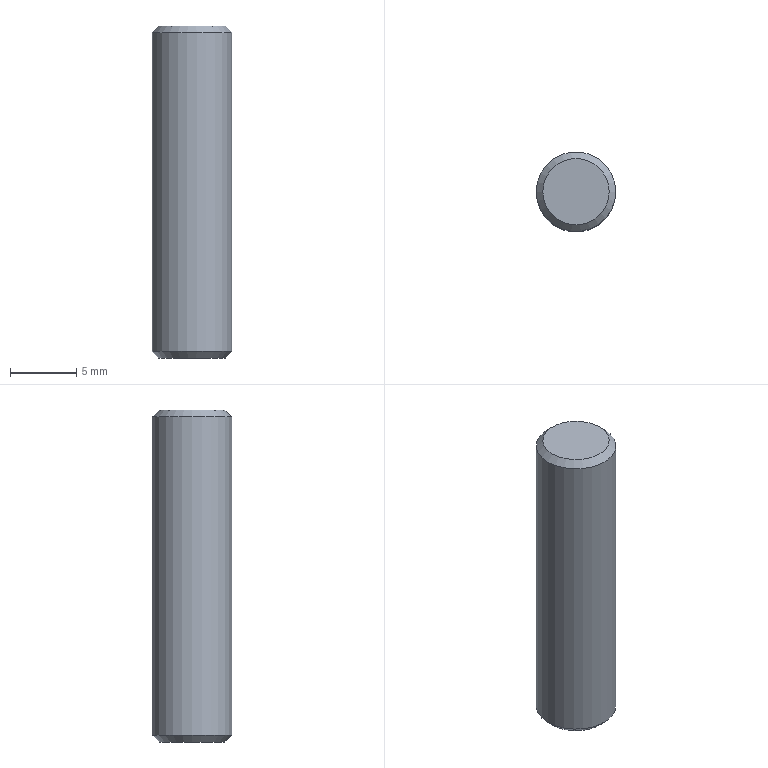Part | NX | features CHAMFER 2, DATUM_CSYS 2, EXTRUDE 1, SKETCH 1 | 1 solid | 5 faces | box 6 x 6 x 25 mm | volume 702.408 mm3 | plane 2 | cone 2 | cylinder 1 | commonest cylinder face diameters 6 x1
STEP:
#1=CARTESIAN_POINT('',(3.,0.,0.5));
#2=VERTEX_POINT('',#1);
#3=CARTESIAN_POINT('',(0.,0.,0.5));
#4=DIRECTION('',(0.,0.,1.));
#5=DIRECTION('',(1.,0.,0.));
#6=AXIS2_PLACEMENT_3D('',#3,#4,#5);
#7=CIRCLE('',#6,3.);
#8=EDGE_CURVE('',#2,#2,#7,.T.);
#9=ORIENTED_EDGE('',*,*,#8,.T.);
#10=EDGE_LOOP('',(#9));
#11=FACE_BOUND('',#10,.T.);
#12=CARTESIAN_POINT('',(3.,0.,24.5));
#13=VERTEX_POINT('',#12);
#14=CARTESIAN_POINT('',(0.,0.,24.5));
#15=DIRECTION('',(0.,0.,1.));
#16=DIRECTION('',(1.,0.,0.));
#17=AXIS2_PLACEMENT_3D('',#14,#15,#16);
#18=CIRCLE('',#17,3.);
#19=EDGE_CURVE('',#13,#13,#18,.F.);
#20=ORIENTED_EDGE('',*,*,#19,.T.);
#21=EDGE_LOOP('',(#20));
#22=FACE_BOUND('',#21,.T.);
#23=CARTESIAN_POINT('',(0.,0.,25.));
#24=DIRECTION('',(0.,0.,-1.));
#25=DIRECTION('',(-1.,0.,0.));
#26=AXIS2_PLACEMENT_3D('',#23,#24,#25);
#27=CYLINDRICAL_SURFACE('',#26,3.);
#28=ADVANCED_FACE('',(#11,#22),#27,.T.);
#29=CARTESIAN_POINT('',(2.5,0.,25.));
#30=VERTEX_POINT('',#29);
#31=CARTESIAN_POINT('',(0.,0.,25.));
#32=DIRECTION('',(0.,0.,1.));
#33=DIRECTION('',(1.,0.,0.));
#34=AXIS2_PLACEMENT_3D('',#31,#32,#33);
#35=CIRCLE('',#34,2.5);
#36=EDGE_CURVE('',#30,#30,#35,.T.);
#37=ORIENTED_EDGE('',*,*,#36,.T.);
#38=EDGE_LOOP('',(#37));
#39=FACE_BOUND('',#38,.T.);
#40=CARTESIAN_POINT('',(0.,0.,25.));
#41=DIRECTION('',(0.,0.,1.));
#42=DIRECTION('',(1.,0.,0.));
#43=AXIS2_PLACEMENT_3D('',#40,#41,#42);
#44=PLANE('',#43);
#45=ADVANCED_FACE('',(#39),#44,.T.);
#46=CARTESIAN_POINT('',(2.5,0.,0.));
#47=VERTEX_POINT('',#46);
#48=CARTESIAN_POINT('',(0.,0.,0.));
#49=DIRECTION('',(0.,0.,1.));
#50=DIRECTION('',(1.,0.,0.));
#51=AXIS2_PLACEMENT_3D('',#48,#49,#50);
#52=CIRCLE('',#51,2.5);
#53=EDGE_CURVE('',#47,#47,#52,.F.);
#54=ORIENTED_EDGE('',*,*,#53,.T.);
#55=EDGE_LOOP('',(#54));
#56=FACE_BOUND('',#55,.T.);
#57=CARTESIAN_POINT('',(0.,0.,0.));
#58=DIRECTION('',(0.,0.,1.));
#59=DIRECTION('',(1.,0.,0.));
#60=AXIS2_PLACEMENT_3D('',#57,#58,#59);
#61=PLANE('',#60);
#62=ADVANCED_FACE('',(#56),#61,.F.);
#63=ORIENTED_EDGE('',*,*,#19,.F.);
#64=EDGE_LOOP('',(#63));
#65=FACE_BOUND('',#64,.T.);
#66=ORIENTED_EDGE('',*,*,#36,.F.);
#67=EDGE_LOOP('',(#66));
#68=FACE_BOUND('',#67,.T.);
#69=CARTESIAN_POINT('',(0.,0.,25.));
#70=DIRECTION('',(0.,0.,-1.));
#71=DIRECTION('',(-1.,0.,0.));
#72=AXIS2_PLACEMENT_3D('',#69,#70,#71);
#73=CONICAL_SURFACE('',#72,2.5,0.7854);
#74=ADVANCED_FACE('',(#65,#68),#73,.T.);
#75=ORIENTED_EDGE('',*,*,#53,.F.);
#76=EDGE_LOOP('',(#75));
#77=FACE_BOUND('',#76,.T.);
#78=ORIENTED_EDGE('',*,*,#8,.F.);
#79=EDGE_LOOP('',(#78));
#80=FACE_BOUND('',#79,.T.);
#81=CARTESIAN_POINT('',(0.,0.,0.5));
#82=DIRECTION('',(0.,0.,1.));
#83=DIRECTION('',(1.,0.,0.));
#84=AXIS2_PLACEMENT_3D('',#81,#82,#83);
#85=CONICAL_SURFACE('',#84,3.,0.7854);
#86=ADVANCED_FACE('',(#77,#80),#85,.T.);
#87=CLOSED_SHELL('',(#28,#45,#62,#74,#86));
#88=MANIFOLD_SOLID_BREP('',#87);
#89=(LENGTH_UNIT()NAMED_UNIT(*)SI_UNIT(.MILLI.,.METRE.));
#90=UNCERTAINTY_MEASURE_WITH_UNIT(LENGTH_MEASURE(0.00001),#89,'','');
#91=(NAMED_UNIT(*)PLANE_ANGLE_UNIT()SI_UNIT($,.RADIAN.));
#92=(NAMED_UNIT(*)SI_UNIT($,.STERADIAN.)SOLID_ANGLE_UNIT());
#93=(GEOMETRIC_REPRESENTATION_CONTEXT(3)GLOBAL_UNCERTAINTY_ASSIGNED_CONTEXT((#90))GLOBAL_UNIT_ASSIGNED_CONTEXT((#89,#91,#92))REPRESENTATION_CONTEXT('',''));
#94=ADVANCED_BREP_SHAPE_REPRESENTATION('',(#88),#93);